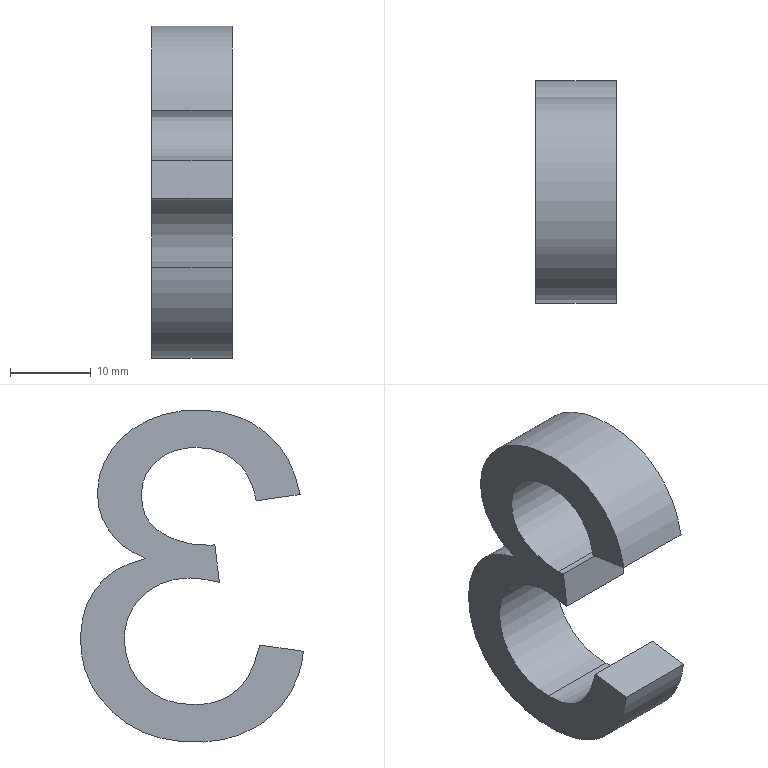Part | NX | features solid 2 | 1 solid | 14 faces | box 10 x 27.61 x 41.147 mm | volume 4412 mm3 | spline 9 | plane 5
STEP:
#1=CARTESIAN_POINT('',(2250.,-298.625,-587.676));
#2=VERTEX_POINT('',#1);
#3=CARTESIAN_POINT('',(2250.,-302.8,-579.522));
#4=VERTEX_POINT('',#3);
#5=CARTESIAN_POINT('',(2250.,-298.625,-587.676));
#6=CARTESIAN_POINT('',(2250.,-301.072,-585.595));
#7=CARTESIAN_POINT('',(2250.,-302.463,-582.872));
#8=CARTESIAN_POINT('',(2250.,-302.8,-579.522));
#9=B_SPLINE_CURVE_WITH_KNOTS('',3,(#5,#6,#7,#8),.UNSPECIFIED.,.F.,.F.,(4,4),(0.,0.04757),.PIECEWISE_BEZIER_KNOTS.);
#10=EDGE_CURVE('',#2,#4,#9,.T.);
#11=ORIENTED_EDGE('',*,*,#10,.F.);
#12=CARTESIAN_POINT('',(2260.,-298.625,-587.676));
#13=VERTEX_POINT('',#12);
#14=CARTESIAN_POINT('',(2260.,-298.625,-587.676));
#15=DIRECTION('',(-1.,0.,0.));
#16=VECTOR('',#15,1000.);
#17=LINE('',#14,#16);
#18=EDGE_CURVE('',#13,#2,#17,.T.);
#19=ORIENTED_EDGE('',*,*,#18,.F.);
#20=CARTESIAN_POINT('',(2260.,-302.8,-579.522));
#21=VERTEX_POINT('',#20);
#22=CARTESIAN_POINT('',(2260.,-298.625,-587.676));
#23=CARTESIAN_POINT('',(2260.,-301.072,-585.595));
#24=CARTESIAN_POINT('',(2260.,-302.463,-582.872));
#25=CARTESIAN_POINT('',(2260.,-302.8,-579.522));
#26=B_SPLINE_CURVE_WITH_KNOTS('',3,(#22,#23,#24,#25),.UNSPECIFIED.,.F.,.F.,(4,4),(0.,0.04757),.PIECEWISE_BEZIER_KNOTS.);
#27=EDGE_CURVE('',#13,#21,#26,.T.);
#28=ORIENTED_EDGE('',*,*,#27,.T.);
#29=CARTESIAN_POINT('',(2260.,-302.8,-579.522));
#30=DIRECTION('',(-1.,0.,0.));
#31=VECTOR('',#30,1000.);
#32=LINE('',#29,#31);
#33=EDGE_CURVE('',#21,#4,#32,.T.);
#34=ORIENTED_EDGE('',*,*,#33,.T.);
#35=EDGE_LOOP('',(#11,#19,#28,#34));
#36=FACE_BOUND('',#35,.T.);
#37=CARTESIAN_POINT('',(2260.,-298.625,-587.676));
#38=CARTESIAN_POINT('',(2250.,-298.625,-587.676));
#39=CARTESIAN_POINT('',(2260.,-301.072,-585.595));
#40=CARTESIAN_POINT('',(2250.,-301.072,-585.595));
#41=CARTESIAN_POINT('',(2260.,-302.463,-582.872));
#42=CARTESIAN_POINT('',(2250.,-302.463,-582.872));
#43=CARTESIAN_POINT('',(2260.,-302.8,-579.522));
#44=CARTESIAN_POINT('',(2250.,-302.8,-579.522));
#45=B_SPLINE_SURFACE_WITH_KNOTS('',3,1,((#37,#38),(#39,#40),(#41,#42),(#43,#44)),.SURF_OF_LINEAR_EXTRUSION.,.F.,.F.,.F.,(4,4),(2,2),(0.,0.04757),(0.,1.),.PIECEWISE_BEZIER_KNOTS.);
#46=ADVANCED_FACE('',(#36),#45,.T.);
#47=CARTESIAN_POINT('',(2250.,-297.37,-578.742));
#48=VERTEX_POINT('',#47);
#49=CARTESIAN_POINT('',(2250.,-302.8,-579.522));
#50=CARTESIAN_POINT('',(2250.,-300.99,-579.262));
#51=CARTESIAN_POINT('',(2250.,-299.18,-579.002));
#52=CARTESIAN_POINT('',(2250.,-297.37,-578.742));
#53=B_SPLINE_CURVE_WITH_KNOTS('',3,(#49,#50,#51,#52),.UNSPECIFIED.,.F.,.F.,(4,4),(0.04757,0.07533),.PIECEWISE_BEZIER_KNOTS.);
#54=EDGE_CURVE('',#4,#48,#53,.T.);
#55=ORIENTED_EDGE('',*,*,#54,.F.);
#56=ORIENTED_EDGE('',*,*,#33,.F.);
#57=CARTESIAN_POINT('',(2260.,-297.37,-578.742));
#58=VERTEX_POINT('',#57);
#59=CARTESIAN_POINT('',(2260.,-302.8,-579.522));
#60=CARTESIAN_POINT('',(2260.,-300.99,-579.262));
#61=CARTESIAN_POINT('',(2260.,-299.18,-579.002));
#62=CARTESIAN_POINT('',(2260.,-297.37,-578.742));
#63=B_SPLINE_CURVE_WITH_KNOTS('',3,(#59,#60,#61,#62),.UNSPECIFIED.,.F.,.F.,(4,4),(0.04757,0.07533),.PIECEWISE_BEZIER_KNOTS.);
#64=EDGE_CURVE('',#21,#58,#63,.T.);
#65=ORIENTED_EDGE('',*,*,#64,.T.);
#66=CARTESIAN_POINT('',(2260.,-297.37,-578.742));
#67=DIRECTION('',(-1.,0.,0.));
#68=VECTOR('',#67,1000.);
#69=LINE('',#66,#68);
#70=EDGE_CURVE('',#58,#48,#69,.T.);
#71=ORIENTED_EDGE('',*,*,#70,.T.);
#72=EDGE_LOOP('',(#55,#56,#65,#71));
#73=FACE_BOUND('',#72,.T.);
#74=CARTESIAN_POINT('',(2260.,-302.8,-579.522));
#75=DIRECTION('',(0.,-0.1422,0.9898));
#76=DIRECTION('',(0.,-0.9898,-0.1422));
#77=AXIS2_PLACEMENT_3D('',#74,#75,#76);
#78=PLANE('',#77);
#79=ADVANCED_FACE('',(#73),#78,.T.);
#80=CARTESIAN_POINT('',(2250.,-289.232,-586.115));
#81=VERTEX_POINT('',#80);
#82=CARTESIAN_POINT('',(2250.,-297.37,-578.742));
#83=CARTESIAN_POINT('',(2250.,-296.789,-581.388));
#84=CARTESIAN_POINT('',(2250.,-295.825,-583.285));
#85=CARTESIAN_POINT('',(2250.,-293.123,-585.583));
#86=CARTESIAN_POINT('',(2250.,-291.374,-586.145));
#87=CARTESIAN_POINT('',(2250.,-289.232,-586.115));
#88=B_SPLINE_CURVE_WITH_KNOTS('',3,(#82,#83,#84,#85,#86,#87),.UNSPECIFIED.,.F.,.F.,(4,2,4),(0.07533,0.1081,0.1418),.UNSPECIFIED.);
#89=EDGE_CURVE('',#48,#81,#88,.T.);
#90=ORIENTED_EDGE('',*,*,#89,.F.);
#91=ORIENTED_EDGE('',*,*,#70,.F.);
#92=CARTESIAN_POINT('',(2260.,-289.232,-586.115));
#93=VERTEX_POINT('',#92);
#94=CARTESIAN_POINT('',(2260.,-297.37,-578.742));
#95=CARTESIAN_POINT('',(2260.,-296.789,-581.388));
#96=CARTESIAN_POINT('',(2260.,-295.825,-583.285));
#97=CARTESIAN_POINT('',(2260.,-293.123,-585.583));
#98=CARTESIAN_POINT('',(2260.,-291.374,-586.145));
#99=CARTESIAN_POINT('',(2260.,-289.232,-586.115));
#100=B_SPLINE_CURVE_WITH_KNOTS('',3,(#94,#95,#96,#97,#98,#99),.UNSPECIFIED.,.F.,.F.,(4,2,4),(0.07533,0.1081,0.1418),.UNSPECIFIED.);
#101=EDGE_CURVE('',#58,#93,#100,.T.);
#102=ORIENTED_EDGE('',*,*,#101,.T.);
#103=CARTESIAN_POINT('',(2260.,-289.232,-586.115));
#104=DIRECTION('',(-1.,0.,0.));
#105=VECTOR('',#104,1000.);
#106=LINE('',#103,#105);
#107=EDGE_CURVE('',#93,#81,#106,.T.);
#108=ORIENTED_EDGE('',*,*,#107,.T.);
#109=EDGE_LOOP('',(#90,#91,#102,#108));
#110=FACE_BOUND('',#109,.T.);
#111=CARTESIAN_POINT('',(2260.,-297.37,-578.742));
#112=CARTESIAN_POINT('',(2250.,-297.37,-578.742));
#113=CARTESIAN_POINT('',(2260.,-296.19,-584.115));
#114=CARTESIAN_POINT('',(2250.,-296.19,-584.115));
#115=CARTESIAN_POINT('',(2260.,-293.452,-586.175));
#116=CARTESIAN_POINT('',(2250.,-293.452,-586.175));
#117=CARTESIAN_POINT('',(2260.,-289.232,-586.115));
#118=CARTESIAN_POINT('',(2250.,-289.232,-586.115));
#119=B_SPLINE_SURFACE_WITH_KNOTS('',3,1,((#111,#112),(#113,#114),(#115,#116),(#117,#118)),.SURF_OF_LINEAR_EXTRUSION.,.F.,.F.,.F.,(4,4),(2,2),(0.07533,0.1418),(0.,1.),.PIECEWISE_BEZIER_KNOTS.);
#120=ADVANCED_FACE('',(#110),#119,.T.);
#121=CARTESIAN_POINT('',(2250.,-288.789,-570.436));
#122=VERTEX_POINT('',#121);
#123=CARTESIAN_POINT('',(2250.,-289.232,-586.115));
#124=CARTESIAN_POINT('',(2250.,-286.678,-586.145));
#125=CARTESIAN_POINT('',(2250.,-284.613,-585.365));
#126=CARTESIAN_POINT('',(2250.,-283.014,-583.813));
#127=CARTESIAN_POINT('',(2250.,-281.416,-582.26));
#128=CARTESIAN_POINT('',(2250.,-280.636,-580.348));
#129=CARTESIAN_POINT('',(2250.,-280.636,-575.836));
#130=CARTESIAN_POINT('',(2250.,-281.385,-574.031));
#131=CARTESIAN_POINT('',(2250.,-284.451,-571.208));
#132=CARTESIAN_POINT('',(2250.,-286.418,-570.467));
#133=CARTESIAN_POINT('',(2250.,-288.789,-570.436));
#134=B_SPLINE_CURVE_WITH_KNOTS('',3,(#123,#124,#125,#126,#127,#128,#129,#130,#131,#132,#133),.UNSPECIFIED.,.F.,.F.,(4,3,2,2,4),(0.1418,0.1776,0.2115,0.243,0.2739),.UNSPECIFIED.);
#135=EDGE_CURVE('',#81,#122,#134,.T.);
#136=ORIENTED_EDGE('',*,*,#135,.F.);
#137=ORIENTED_EDGE('',*,*,#107,.F.);
#138=CARTESIAN_POINT('',(2260.,-288.789,-570.436));
#139=VERTEX_POINT('',#138);
#140=CARTESIAN_POINT('',(2260.,-289.232,-586.115));
#141=CARTESIAN_POINT('',(2260.,-286.678,-586.145));
#142=CARTESIAN_POINT('',(2260.,-284.613,-585.365));
#143=CARTESIAN_POINT('',(2260.,-283.014,-583.813));
#144=CARTESIAN_POINT('',(2260.,-281.416,-582.26));
#145=CARTESIAN_POINT('',(2260.,-280.636,-580.348));
#146=CARTESIAN_POINT('',(2260.,-280.636,-575.836));
#147=CARTESIAN_POINT('',(2260.,-281.385,-574.031));
#148=CARTESIAN_POINT('',(2260.,-284.451,-571.208));
#149=CARTESIAN_POINT('',(2260.,-286.418,-570.467));
#150=CARTESIAN_POINT('',(2260.,-288.789,-570.436));
#151=B_SPLINE_CURVE_WITH_KNOTS('',3,(#140,#141,#142,#143,#144,#145,#146,#147,#148,#149,#150),.UNSPECIFIED.,.F.,.F.,(4,3,2,2,4),(0.1418,0.1776,0.2115,0.243,0.2739),.UNSPECIFIED.);
#152=EDGE_CURVE('',#93,#139,#151,.T.);
#153=ORIENTED_EDGE('',*,*,#152,.T.);
#154=CARTESIAN_POINT('',(2260.,-288.789,-570.436));
#155=DIRECTION('',(-1.,0.,0.));
#156=VECTOR('',#155,1000.);
#157=LINE('',#154,#156);
#158=EDGE_CURVE('',#139,#122,#157,.T.);
#159=ORIENTED_EDGE('',*,*,#158,.T.);
#160=EDGE_LOOP('',(#136,#137,#153,#159));
#161=FACE_BOUND('',#160,.T.);
#162=CARTESIAN_POINT('',(2260.,-289.232,-586.115));
#163=CARTESIAN_POINT('',(2250.,-289.232,-586.115));
#164=CARTESIAN_POINT('',(2260.,-286.874,-586.143));
#165=CARTESIAN_POINT('',(2250.,-286.874,-586.143));
#166=CARTESIAN_POINT('',(2260.,-283.972,-585.165));
#167=CARTESIAN_POINT('',(2250.,-283.972,-585.165));
#168=CARTESIAN_POINT('',(2260.,-281.259,-581.812));
#169=CARTESIAN_POINT('',(2250.,-281.259,-581.812));
#170=CARTESIAN_POINT('',(2260.,-280.613,-579.348));
#171=CARTESIAN_POINT('',(2250.,-280.613,-579.348));
#172=CARTESIAN_POINT('',(2260.,-280.632,-577.039));
#173=CARTESIAN_POINT('',(2250.,-280.632,-577.039));
#174=CARTESIAN_POINT('',(2260.,-281.071,-574.988));
#175=CARTESIAN_POINT('',(2250.,-281.071,-574.988));
#176=CARTESIAN_POINT('',(2260.,-282.446,-572.761));
#177=CARTESIAN_POINT('',(2250.,-282.446,-572.761));
#178=CARTESIAN_POINT('',(2260.,-285.243,-570.874));
#179=CARTESIAN_POINT('',(2250.,-285.243,-570.874));
#180=CARTESIAN_POINT('',(2260.,-287.524,-570.452));
#181=CARTESIAN_POINT('',(2250.,-287.524,-570.452));
#182=CARTESIAN_POINT('',(2260.,-288.789,-570.436));
#183=CARTESIAN_POINT('',(2250.,-288.789,-570.436));
#184=B_SPLINE_SURFACE_WITH_KNOTS('',3,1,((#162,#163),(#164,#165),(#166,#167),(#168,#169),(#170,#171),(#172,#173),(#174,#175),(#176,#177),(#178,#179),(#180,#181),(#182,#183)),.SURF_OF_LINEAR_EXTRUSION.,.F.,.F.,.F.,(4,1,1,1,1,1,1,1,4),(2,2),(0.1418,0.1748,0.1914,0.2079,0.2161,0.2244,0.2409,0.2574,0.2739),(0.,1.),.UNSPECIFIED.);
#185=ADVANCED_FACE('',(#161),#184,.T.);
#186=CARTESIAN_POINT('',(2250.,-292.398,-570.971));
#187=VERTEX_POINT('',#186);
#188=CARTESIAN_POINT('',(2250.,-288.789,-570.436));
#189=CARTESIAN_POINT('',(2250.,-289.752,-570.467));
#190=CARTESIAN_POINT('',(2250.,-290.961,-570.635));
#191=CARTESIAN_POINT('',(2250.,-292.398,-570.971));
#192=B_SPLINE_CURVE_WITH_KNOTS('',3,(#188,#189,#190,#191),.UNSPECIFIED.,.F.,.F.,(4,4),(0.2739,0.2929),.PIECEWISE_BEZIER_KNOTS.);
#193=EDGE_CURVE('',#122,#187,#192,.T.);
#194=ORIENTED_EDGE('',*,*,#193,.F.);
#195=ORIENTED_EDGE('',*,*,#158,.F.);
#196=CARTESIAN_POINT('',(2260.,-292.398,-570.971));
#197=VERTEX_POINT('',#196);
#198=CARTESIAN_POINT('',(2260.,-288.789,-570.436));
#199=CARTESIAN_POINT('',(2260.,-289.752,-570.467));
#200=CARTESIAN_POINT('',(2260.,-290.961,-570.635));
#201=CARTESIAN_POINT('',(2260.,-292.398,-570.971));
#202=B_SPLINE_CURVE_WITH_KNOTS('',3,(#198,#199,#200,#201),.UNSPECIFIED.,.F.,.F.,(4,4),(0.2739,0.2929),.PIECEWISE_BEZIER_KNOTS.);
#203=EDGE_CURVE('',#139,#197,#202,.T.);
#204=ORIENTED_EDGE('',*,*,#203,.T.);
#205=CARTESIAN_POINT('',(2260.,-292.398,-570.971));
#206=DIRECTION('',(-1.,0.,0.));
#207=VECTOR('',#206,1000.);
#208=LINE('',#205,#207);
#209=EDGE_CURVE('',#197,#187,#208,.T.);
#210=ORIENTED_EDGE('',*,*,#209,.T.);
#211=EDGE_LOOP('',(#194,#195,#204,#210));
#212=FACE_BOUND('',#211,.T.);
#213=CARTESIAN_POINT('',(2260.,-288.789,-570.436));
#214=CARTESIAN_POINT('',(2250.,-288.789,-570.436));
#215=CARTESIAN_POINT('',(2260.,-289.752,-570.467));
#216=CARTESIAN_POINT('',(2250.,-289.752,-570.467));
#217=CARTESIAN_POINT('',(2260.,-290.961,-570.635));
#218=CARTESIAN_POINT('',(2250.,-290.961,-570.635));
#219=CARTESIAN_POINT('',(2260.,-292.398,-570.971));
#220=CARTESIAN_POINT('',(2250.,-292.398,-570.971));
#221=B_SPLINE_SURFACE_WITH_KNOTS('',3,1,((#213,#214),(#215,#216),(#217,#218),(#219,#220)),.SURF_OF_LINEAR_EXTRUSION.,.F.,.F.,.F.,(4,4),(2,2),(0.2739,0.2929),(0.,1.),.PIECEWISE_BEZIER_KNOTS.);
#222=ADVANCED_FACE('',(#212),#221,.T.);
#223=CARTESIAN_POINT('',(2250.,-291.817,-566.321));
#224=VERTEX_POINT('',#223);
#225=CARTESIAN_POINT('',(2250.,-292.398,-570.971));
#226=CARTESIAN_POINT('',(2250.,-292.205,-569.421));
#227=CARTESIAN_POINT('',(2250.,-292.011,-567.871));
#228=CARTESIAN_POINT('',(2250.,-291.817,-566.321));
#229=B_SPLINE_CURVE_WITH_KNOTS('',3,(#225,#226,#227,#228),.UNSPECIFIED.,.F.,.F.,(4,4),(0.2929,0.3173),.PIECEWISE_BEZIER_KNOTS.);
#230=EDGE_CURVE('',#187,#224,#229,.T.);
#231=ORIENTED_EDGE('',*,*,#230,.F.);
#232=ORIENTED_EDGE('',*,*,#209,.F.);
#233=CARTESIAN_POINT('',(2260.,-291.817,-566.321));
#234=VERTEX_POINT('',#233);
#235=CARTESIAN_POINT('',(2260.,-292.398,-570.971));
#236=CARTESIAN_POINT('',(2260.,-292.205,-569.421));
#237=CARTESIAN_POINT('',(2260.,-292.011,-567.871));
#238=CARTESIAN_POINT('',(2260.,-291.817,-566.321));
#239=B_SPLINE_CURVE_WITH_KNOTS('',3,(#235,#236,#237,#238),.UNSPECIFIED.,.F.,.F.,(4,4),(0.2929,0.3173),.PIECEWISE_BEZIER_KNOTS.);
#240=EDGE_CURVE('',#197,#234,#239,.T.);
#241=ORIENTED_EDGE('',*,*,#240,.T.);
#242=CARTESIAN_POINT('',(2260.,-291.817,-566.321));
#243=DIRECTION('',(-1.,0.,0.));
#244=VECTOR('',#243,1000.);
#245=LINE('',#242,#244);
#246=EDGE_CURVE('',#234,#224,#245,.T.);
#247=ORIENTED_EDGE('',*,*,#246,.T.);
#248=EDGE_LOOP('',(#231,#232,#241,#247));
#249=FACE_BOUND('',#248,.T.);
#250=CARTESIAN_POINT('',(2260.,-292.398,-570.971));
#251=DIRECTION('',(0.,-0.9923,0.124));
#252=DIRECTION('',(0.,-0.124,-0.9923));
#253=AXIS2_PLACEMENT_3D('',#250,#251,#252);
#254=PLANE('',#253);
#255=ADVANCED_FACE('',(#249),#254,.T.);
#256=CARTESIAN_POINT('',(2250.,-291.007,-566.382));
#257=VERTEX_POINT('',#256);
#258=CARTESIAN_POINT('',(2250.,-291.817,-566.321));
#259=CARTESIAN_POINT('',(2250.,-291.481,-566.382));
#260=CARTESIAN_POINT('',(2250.,-291.221,-566.413));
#261=CARTESIAN_POINT('',(2250.,-291.007,-566.382));
#262=B_SPLINE_CURVE_WITH_KNOTS('',3,(#258,#259,#260,#261),.UNSPECIFIED.,.F.,.F.,(4,4),(0.3173,0.3215),.PIECEWISE_BEZIER_KNOTS.);
#263=EDGE_CURVE('',#224,#257,#262,.T.);
#264=ORIENTED_EDGE('',*,*,#263,.F.);
#265=ORIENTED_EDGE('',*,*,#246,.F.);
#266=CARTESIAN_POINT('',(2260.,-291.007,-566.382));
#267=VERTEX_POINT('',#266);
#268=CARTESIAN_POINT('',(2260.,-291.817,-566.321));
#269=CARTESIAN_POINT('',(2260.,-291.481,-566.382));
#270=CARTESIAN_POINT('',(2260.,-291.221,-566.413));
#271=CARTESIAN_POINT('',(2260.,-291.007,-566.382));
#272=B_SPLINE_CURVE_WITH_KNOTS('',3,(#268,#269,#270,#271),.UNSPECIFIED.,.F.,.F.,(4,4),(0.3173,0.3215),.PIECEWISE_BEZIER_KNOTS.);
#273=EDGE_CURVE('',#234,#267,#272,.T.);
#274=ORIENTED_EDGE('',*,*,#273,.T.);
#275=CARTESIAN_POINT('',(2260.,-291.007,-566.382));
#276=DIRECTION('',(-1.,0.,0.));
#277=VECTOR('',#276,1000.);
#278=LINE('',#275,#277);
#279=EDGE_CURVE('',#267,#257,#278,.T.);
#280=ORIENTED_EDGE('',*,*,#279,.T.);
#281=EDGE_LOOP('',(#264,#265,#274,#280));
#282=FACE_BOUND('',#281,.T.);
#283=CARTESIAN_POINT('',(2260.,-291.817,-566.321));
#284=CARTESIAN_POINT('',(2250.,-291.817,-566.321));
#285=CARTESIAN_POINT('',(2260.,-291.481,-566.382));
#286=CARTESIAN_POINT('',(2250.,-291.481,-566.382));
#287=CARTESIAN_POINT('',(2260.,-291.221,-566.413));
#288=CARTESIAN_POINT('',(2250.,-291.221,-566.413));
#289=CARTESIAN_POINT('',(2260.,-291.007,-566.382));
#290=CARTESIAN_POINT('',(2250.,-291.007,-566.382));
#291=B_SPLINE_SURFACE_WITH_KNOTS('',3,1,((#283,#284),(#285,#286),(#287,#288),(#289,#290)),.SURF_OF_LINEAR_EXTRUSION.,.F.,.F.,.F.,(4,4),(2,2),(0.3173,0.3215),(0.,1.),.PIECEWISE_BEZIER_KNOTS.);
#292=ADVANCED_FACE('',(#282),#291,.T.);
#293=CARTESIAN_POINT('',(2250.,-289.492,-554.268));
#294=VERTEX_POINT('',#293);
#295=CARTESIAN_POINT('',(2250.,-291.007,-566.382));
#296=CARTESIAN_POINT('',(2250.,-288.865,-566.413));
#297=CARTESIAN_POINT('',(2250.,-286.968,-565.908));
#298=CARTESIAN_POINT('',(2250.,-285.247,-564.866));
#299=CARTESIAN_POINT('',(2250.,-283.557,-563.843));
#300=CARTESIAN_POINT('',(2250.,-282.731,-562.268));
#301=CARTESIAN_POINT('',(2250.,-282.731,-558.474));
#302=CARTESIAN_POINT('',(2250.,-283.358,-557.067));
#303=CARTESIAN_POINT('',(2250.,-284.62,-555.959));
#304=CARTESIAN_POINT('',(2250.,-285.867,-554.864));
#305=CARTESIAN_POINT('',(2250.,-287.504,-554.298));
#306=CARTESIAN_POINT('',(2250.,-289.492,-554.268));
#307=B_SPLINE_CURVE_WITH_KNOTS('',3,(#295,#296,#297,#298,#299,#300,#301,#302,#303,#304,#305,#306),.UNSPECIFIED.,.F.,.F.,(4,3,2,3,4),(0.3215,0.3528,0.3821,0.4047,0.4319),.UNSPECIFIED.);
#308=EDGE_CURVE('',#257,#294,#307,.T.);
#309=ORIENTED_EDGE('',*,*,#308,.F.);
#310=ORIENTED_EDGE('',*,*,#279,.F.);
#311=CARTESIAN_POINT('',(2260.,-289.492,-554.268));
#312=VERTEX_POINT('',#311);
#313=CARTESIAN_POINT('',(2260.,-291.007,-566.382));
#314=CARTESIAN_POINT('',(2260.,-288.865,-566.413));
#315=CARTESIAN_POINT('',(2260.,-286.968,-565.908));
#316=CARTESIAN_POINT('',(2260.,-285.247,-564.866));
#317=CARTESIAN_POINT('',(2260.,-283.557,-563.843));
#318=CARTESIAN_POINT('',(2260.,-282.731,-562.268));
#319=CARTESIAN_POINT('',(2260.,-282.731,-558.474));
#320=CARTESIAN_POINT('',(2260.,-283.358,-557.067));
#321=CARTESIAN_POINT('',(2260.,-284.62,-555.959));
#322=CARTESIAN_POINT('',(2260.,-285.867,-554.864));
#323=CARTESIAN_POINT('',(2260.,-287.504,-554.298));
#324=CARTESIAN_POINT('',(2260.,-289.492,-554.268));
#325=B_SPLINE_CURVE_WITH_KNOTS('',3,(#313,#314,#315,#316,#317,#318,#319,#320,#321,#322,#323,#324),.UNSPECIFIED.,.F.,.F.,(4,3,2,3,4),(0.3215,0.3528,0.3821,0.4047,0.4319),.UNSPECIFIED.);
#326=EDGE_CURVE('',#267,#312,#325,.T.);
#327=ORIENTED_EDGE('',*,*,#326,.T.);
#328=CARTESIAN_POINT('',(2260.,-289.492,-554.268));
#329=DIRECTION('',(-1.,0.,0.));
#330=VECTOR('',#329,1000.);
#331=LINE('',#328,#330);
#332=EDGE_CURVE('',#312,#294,#331,.T.);
#333=ORIENTED_EDGE('',*,*,#332,.T.);
#334=EDGE_LOOP('',(#309,#310,#327,#333));
#335=FACE_BOUND('',#334,.T.);
#336=CARTESIAN_POINT('',(2260.,-291.007,-566.382));
#337=CARTESIAN_POINT('',(2250.,-291.007,-566.382));
#338=CARTESIAN_POINT('',(2260.,-290.063,-566.396));
#339=CARTESIAN_POINT('',(2250.,-290.063,-566.396));
#340=CARTESIAN_POINT('',(2260.,-288.271,-566.21));
#341=CARTESIAN_POINT('',(2250.,-288.271,-566.21));
#342=CARTESIAN_POINT('',(2260.,-285.84,-565.338));
#343=CARTESIAN_POINT('',(2250.,-285.84,-565.338));
#344=CARTESIAN_POINT('',(2260.,-283.591,-563.735));
#345=CARTESIAN_POINT('',(2250.,-283.591,-563.735));
#346=CARTESIAN_POINT('',(2260.,-282.803,-561.792));
#347=CARTESIAN_POINT('',(2250.,-282.803,-561.792));
#348=CARTESIAN_POINT('',(2260.,-282.683,-559.786));
#349=CARTESIAN_POINT('',(2250.,-282.683,-559.786));
#350=CARTESIAN_POINT('',(2260.,-282.932,-558.358));
#351=CARTESIAN_POINT('',(2250.,-282.932,-558.358));
#352=CARTESIAN_POINT('',(2260.,-283.442,-557.302));
#353=CARTESIAN_POINT('',(2250.,-283.442,-557.302));
#354=CARTESIAN_POINT('',(2260.,-284.014,-556.543));
#355=CARTESIAN_POINT('',(2250.,-284.014,-556.543));
#356=CARTESIAN_POINT('',(2260.,-284.753,-555.803));
#357=CARTESIAN_POINT('',(2250.,-284.753,-555.803));
#358=CARTESIAN_POINT('',(2260.,-285.547,-555.242));
#359=CARTESIAN_POINT('',(2250.,-285.547,-555.242));
#360=CARTESIAN_POINT('',(2260.,-287.117,-554.504));
#361=CARTESIAN_POINT('',(2250.,-287.117,-554.504));
#362=CARTESIAN_POINT('',(2260.,-288.485,-554.283));
#363=CARTESIAN_POINT('',(2250.,-288.485,-554.283));
#364=CARTESIAN_POINT('',(2260.,-289.492,-554.268));
#365=CARTESIAN_POINT('',(2250.,-289.492,-554.268));
#366=B_SPLINE_SURFACE_WITH_KNOTS('',3,1,((#336,#337),(#338,#339),(#340,#341),(#342,#343),(#344,#345),(#346,#347),(#348,#349),(#350,#351),(#352,#353),(#354,#355),(#356,#357),(#358,#359),(#360,#361),(#362,#363),(#364,#365)),.SURF_OF_LINEAR_EXTRUSION.,.F.,.F.,.F.,(4,1,1,1,1,1,1,1,1,1,1,1,4),(2,2),(0.3215,0.3353,0.3491,0.3629,0.3767,0.3836,0.3905,0.3974,0.4009,0.4043,0.4112,0.4181,0.4319),(0.,1.),.UNSPECIFIED.);
#367=ADVANCED_FACE('',(#335),#366,.T.);
#368=CARTESIAN_POINT('',(2250.,-296.941,-560.876));
#369=VERTEX_POINT('',#368);
#370=CARTESIAN_POINT('',(2250.,-289.492,-554.268));
#371=CARTESIAN_POINT('',(2250.,-291.45,-554.298));
#372=CARTESIAN_POINT('',(2250.,-293.102,-554.864));
#373=CARTESIAN_POINT('',(2250.,-294.407,-555.963));
#374=CARTESIAN_POINT('',(2250.,-295.718,-557.067));
#375=CARTESIAN_POINT('',(2250.,-296.574,-558.688));
#376=CARTESIAN_POINT('',(2250.,-296.941,-560.876));
#377=B_SPLINE_CURVE_WITH_KNOTS('',3,(#370,#371,#372,#373,#374,#375,#376),.UNSPECIFIED.,.F.,.F.,(4,3,4),(0.4319,0.4594,0.4886),.PIECEWISE_BEZIER_KNOTS.);
#378=EDGE_CURVE('',#294,#369,#377,.T.);
#379=ORIENTED_EDGE('',*,*,#378,.F.);
#380=ORIENTED_EDGE('',*,*,#332,.F.);
#381=CARTESIAN_POINT('',(2260.,-296.941,-560.876));
#382=VERTEX_POINT('',#381);
#383=CARTESIAN_POINT('',(2260.,-289.492,-554.268));
#384=CARTESIAN_POINT('',(2260.,-291.45,-554.298));
#385=CARTESIAN_POINT('',(2260.,-293.102,-554.864));
#386=CARTESIAN_POINT('',(2260.,-294.407,-555.963));
#387=CARTESIAN_POINT('',(2260.,-295.718,-557.067));
#388=CARTESIAN_POINT('',(2260.,-296.574,-558.688));
#389=CARTESIAN_POINT('',(2260.,-296.941,-560.876));
#390=B_SPLINE_CURVE_WITH_KNOTS('',3,(#383,#384,#385,#386,#387,#388,#389),.UNSPECIFIED.,.F.,.F.,(4,3,4),(0.4319,0.4594,0.4886),.PIECEWISE_BEZIER_KNOTS.);
#391=EDGE_CURVE('',#312,#382,#390,.T.);
#392=ORIENTED_EDGE('',*,*,#391,.T.);
#393=CARTESIAN_POINT('',(2260.,-296.941,-560.876));
#394=DIRECTION('',(-1.,0.,0.));
#395=VECTOR('',#394,1000.);
#396=LINE('',#393,#395);
#397=EDGE_CURVE('',#382,#369,#396,.T.);
#398=ORIENTED_EDGE('',*,*,#397,.T.);
#399=EDGE_LOOP('',(#379,#380,#392,#398));
#400=FACE_BOUND('',#399,.T.);
#401=CARTESIAN_POINT('',(2260.,-289.492,-554.268));
#402=CARTESIAN_POINT('',(2250.,-289.492,-554.268));
#403=CARTESIAN_POINT('',(2260.,-290.503,-554.283));
#404=CARTESIAN_POINT('',(2250.,-290.503,-554.283));
#405=CARTESIAN_POINT('',(2260.,-292.354,-554.593));
#406=CARTESIAN_POINT('',(2250.,-292.354,-554.593));
#407=CARTESIAN_POINT('',(2260.,-295.415,-556.41));
#408=CARTESIAN_POINT('',(2250.,-295.415,-556.41));
#409=CARTESIAN_POINT('',(2260.,-296.586,-558.755));
#410=CARTESIAN_POINT('',(2250.,-296.586,-558.755));
#411=CARTESIAN_POINT('',(2260.,-296.941,-560.876));
#412=CARTESIAN_POINT('',(2250.,-296.941,-560.876));
#413=B_SPLINE_SURFACE_WITH_KNOTS('',3,1,((#401,#402),(#403,#404),(#405,#406),(#407,#408),(#409,#410),(#411,#412)),.SURF_OF_LINEAR_EXTRUSION.,.F.,.F.,.F.,(4,1,1,4),(2,2),(0.4319,0.4461,0.4602,0.4886),(0.,1.),.UNSPECIFIED.);
#414=ADVANCED_FACE('',(#400),#413,.T.);
#415=CARTESIAN_POINT('',(2250.,-302.387,-560.096));
#416=VERTEX_POINT('',#415);
#417=CARTESIAN_POINT('',(2250.,-296.941,-560.876));
#418=CARTESIAN_POINT('',(2250.,-298.757,-560.616));
#419=CARTESIAN_POINT('',(2250.,-300.572,-560.356));
#420=CARTESIAN_POINT('',(2250.,-302.387,-560.096));
#421=B_SPLINE_CURVE_WITH_KNOTS('',3,(#417,#418,#419,#420),.UNSPECIFIED.,.F.,.F.,(4,4),(0.4886,0.517),.PIECEWISE_BEZIER_KNOTS.);
#422=EDGE_CURVE('',#369,#416,#421,.T.);
#423=ORIENTED_EDGE('',*,*,#422,.F.);
#424=ORIENTED_EDGE('',*,*,#397,.F.);
#425=CARTESIAN_POINT('',(2260.,-302.387,-560.096));
#426=VERTEX_POINT('',#425);
#427=CARTESIAN_POINT('',(2260.,-296.941,-560.876));
#428=CARTESIAN_POINT('',(2260.,-298.757,-560.616));
#429=CARTESIAN_POINT('',(2260.,-300.572,-560.356));
#430=CARTESIAN_POINT('',(2260.,-302.387,-560.096));
#431=B_SPLINE_CURVE_WITH_KNOTS('',3,(#427,#428,#429,#430),.UNSPECIFIED.,.F.,.F.,(4,4),(0.4886,0.517),.PIECEWISE_BEZIER_KNOTS.);
#432=EDGE_CURVE('',#382,#426,#431,.T.);
#433=ORIENTED_EDGE('',*,*,#432,.T.);
#434=CARTESIAN_POINT('',(2260.,-302.387,-560.096));
#435=DIRECTION('',(-1.,0.,0.));
#436=VECTOR('',#435,1000.);
#437=LINE('',#434,#436);
#438=EDGE_CURVE('',#426,#416,#437,.T.);
#439=ORIENTED_EDGE('',*,*,#438,.T.);
#440=EDGE_LOOP('',(#423,#424,#433,#439));
#441=FACE_BOUND('',#440,.T.);
#442=CARTESIAN_POINT('',(2260.,-296.941,-560.876));
#443=DIRECTION('',(0.,-0.1418,-0.9899));
#444=DIRECTION('',(0.,0.9899,-0.1418));
#445=AXIS2_PLACEMENT_3D('',#442,#443,#444);
#446=PLANE('',#445);
#447=ADVANCED_FACE('',(#441),#446,.T.);
#448=CARTESIAN_POINT('',(2250.,-283.251,-568.034));
#449=VERTEX_POINT('',#448);
#450=CARTESIAN_POINT('',(2250.,-302.387,-560.096));
#451=CARTESIAN_POINT('',(2250.,-301.76,-556.792));
#452=CARTESIAN_POINT('',(2250.,-300.322,-554.222));
#453=CARTESIAN_POINT('',(2250.,-295.832,-550.557));
#454=CARTESIAN_POINT('',(2250.,-293.026,-549.633));
#455=CARTESIAN_POINT('',(2250.,-289.676,-549.633));
#456=CARTESIAN_POINT('',(2250.,-287.351,-549.633));
#457=CARTESIAN_POINT('',(2250.,-285.209,-550.122));
#458=CARTESIAN_POINT('',(2250.,-283.286,-551.05));
#459=CARTESIAN_POINT('',(2250.,-281.339,-551.989));
#460=CARTESIAN_POINT('',(2250.,-279.855,-553.258));
#461=CARTESIAN_POINT('',(2250.,-277.794,-556.488));
#462=CARTESIAN_POINT('',(2250.,-277.286,-558.184));
#463=CARTESIAN_POINT('',(2250.,-277.286,-561.732));
#464=CARTESIAN_POINT('',(2250.,-277.79,-563.277));
#465=CARTESIAN_POINT('',(2250.,-279.779,-566.092));
#466=CARTESIAN_POINT('',(2250.,-281.263,-567.208));
#467=CARTESIAN_POINT('',(2250.,-283.251,-568.034));
#468=B_SPLINE_CURVE_WITH_KNOTS('',3,(#450,#451,#452,#453,#454,#455,#456,#457,#458,#459,#460,#461,#462,#463,#464,#465,#466,#467),.UNSPECIFIED.,.F.,.F.,(4,2,3,3,2,2,2,4),(0.517,0.5636,0.6101,0.6443,0.675,0.706,0.7366,0.7671),.UNSPECIFIED.);
#469=EDGE_CURVE('',#416,#449,#468,.T.);
#470=ORIENTED_EDGE('',*,*,#469,.F.);
#471=ORIENTED_EDGE('',*,*,#438,.F.);
#472=CARTESIAN_POINT('',(2260.,-283.251,-568.034));
#473=VERTEX_POINT('',#472);
#474=CARTESIAN_POINT('',(2260.,-302.387,-560.096));
#475=CARTESIAN_POINT('',(2260.,-301.76,-556.792));
#476=CARTESIAN_POINT('',(2260.,-300.322,-554.222));
#477=CARTESIAN_POINT('',(2260.,-295.832,-550.557));
#478=CARTESIAN_POINT('',(2260.,-293.026,-549.633));
#479=CARTESIAN_POINT('',(2260.,-289.676,-549.633));
#480=CARTESIAN_POINT('',(2260.,-287.351,-549.633));
#481=CARTESIAN_POINT('',(2260.,-285.209,-550.122));
#482=CARTESIAN_POINT('',(2260.,-283.286,-551.05));
#483=CARTESIAN_POINT('',(2260.,-281.339,-551.989));
#484=CARTESIAN_POINT('',(2260.,-279.855,-553.258));
#485=CARTESIAN_POINT('',(2260.,-277.794,-556.488));
#486=CARTESIAN_POINT('',(2260.,-277.286,-558.184));
#487=CARTESIAN_POINT('',(2260.,-277.286,-561.732));
#488=CARTESIAN_POINT('',(2260.,-277.79,-563.277));
#489=CARTESIAN_POINT('',(2260.,-279.779,-566.092));
#490=CARTESIAN_POINT('',(2260.,-281.263,-567.208));
#491=CARTESIAN_POINT('',(2260.,-283.251,-568.034));
#492=B_SPLINE_CURVE_WITH_KNOTS('',3,(#474,#475,#476,#477,#478,#479,#480,#481,#482,#483,#484,#485,#486,#487,#488,#489,#490,#491),.UNSPECIFIED.,.F.,.F.,(4,2,3,3,2,2,2,4),(0.517,0.5636,0.6101,0.6443,0.675,0.706,0.7366,0.7671),.UNSPECIFIED.);
#493=EDGE_CURVE('',#426,#473,#492,.T.);
#494=ORIENTED_EDGE('',*,*,#493,.T.);
#495=CARTESIAN_POINT('',(2260.,-283.251,-568.034));
#496=DIRECTION('',(-1.,0.,0.));
#497=VECTOR('',#496,1000.);
#498=LINE('',#495,#497);
#499=EDGE_CURVE('',#473,#449,#498,.T.);
#500=ORIENTED_EDGE('',*,*,#499,.T.);
#501=EDGE_LOOP('',(#470,#471,#494,#500));
#502=FACE_BOUND('',#501,.T.);
#503=CARTESIAN_POINT('',(2260.,-302.387,-560.096));
#504=CARTESIAN_POINT('',(2250.,-302.387,-560.096));
#505=CARTESIAN_POINT('',(2260.,-301.967,-557.881));
#506=CARTESIAN_POINT('',(2250.,-301.967,-557.881));
#507=CARTESIAN_POINT('',(2260.,-300.799,-555.06));
#508=CARTESIAN_POINT('',(2250.,-300.799,-555.06));
#509=CARTESIAN_POINT('',(2260.,-298.114,-552.264));
#510=CARTESIAN_POINT('',(2250.,-298.114,-552.264));
#511=CARTESIAN_POINT('',(2260.,-295.641,-550.723));
#512=CARTESIAN_POINT('',(2250.,-295.641,-550.723));
#513=CARTESIAN_POINT('',(2260.,-293.275,-549.968));
#514=CARTESIAN_POINT('',(2250.,-293.275,-549.968));
#515=CARTESIAN_POINT('',(2260.,-291.207,-549.673));
#516=CARTESIAN_POINT('',(2250.,-291.207,-549.673));
#517=CARTESIAN_POINT('',(2260.,-288.963,-549.585));
#518=CARTESIAN_POINT('',(2250.,-288.963,-549.585));
#519=CARTESIAN_POINT('',(2260.,-286.429,-549.873));
#520=CARTESIAN_POINT('',(2250.,-286.429,-549.873));
#521=CARTESIAN_POINT('',(2260.,-283.671,-550.749));
#522=CARTESIAN_POINT('',(2250.,-283.671,-550.749));
#523=CARTESIAN_POINT('',(2260.,-280.861,-552.381));
#524=CARTESIAN_POINT('',(2250.,-280.861,-552.381));
#525=CARTESIAN_POINT('',(2260.,-278.218,-555.27));
#526=CARTESIAN_POINT('',(2250.,-278.218,-555.27));
#527=CARTESIAN_POINT('',(2260.,-277.047,-558.857));
#528=CARTESIAN_POINT('',(2250.,-277.047,-558.857));
#529=CARTESIAN_POINT('',(2260.,-277.48,-562.345));
#530=CARTESIAN_POINT('',(2250.,-277.48,-562.345));
#531=CARTESIAN_POINT('',(2260.,-278.954,-565.405));
#532=CARTESIAN_POINT('',(2250.,-278.954,-565.405));
#533=CARTESIAN_POINT('',(2260.,-281.215,-567.189));
#534=CARTESIAN_POINT('',(2250.,-281.215,-567.189));
#535=CARTESIAN_POINT('',(2260.,-283.251,-568.034));
#536=CARTESIAN_POINT('',(2250.,-283.251,-568.034));
#537=B_SPLINE_SURFACE_WITH_KNOTS('',3,1,((#503,#504),(#505,#506),(#507,#508),(#509,#510),(#511,#512),(#513,#514),(#515,#516),(#517,#518),(#519,#520),(#521,#522),(#523,#524),(#525,#526),(#527,#528),(#529,#530),(#531,#532),(#533,#534),(#535,#536)),.SURF_OF_LINEAR_EXTRUSION.,.F.,.F.,.F.,(4,1,1,1,1,1,1,1,1,1,1,1,1,1,4),(2,2),(0.517,0.5483,0.5639,0.5795,0.5952,0.603,0.6108,0.6264,0.642,0.6577,0.6733,0.7046,0.7202,0.7358,0.7671),(0.,1.),.UNSPECIFIED.);
#538=ADVANCED_FACE('',(#502),#537,.T.);
#539=CARTESIAN_POINT('',(2250.,-283.251,-568.034));
#540=CARTESIAN_POINT('',(2250.,-280.681,-568.616));
#541=CARTESIAN_POINT('',(2250.,-278.693,-569.763));
#542=CARTESIAN_POINT('',(2250.,-275.878,-573.25));
#543=CARTESIAN_POINT('',(2250.,-275.19,-575.438));
#544=CARTESIAN_POINT('',(2250.,-275.19,-581.633));
#545=CARTESIAN_POINT('',(2250.,-276.536,-584.646));
#546=CARTESIAN_POINT('',(2250.,-279.214,-587.11));
#547=CARTESIAN_POINT('',(2250.,-281.89,-589.572));
#548=CARTESIAN_POINT('',(2250.,-285.286,-590.78));
#549=CARTESIAN_POINT('',(2250.,-293.102,-590.78));
#550=CARTESIAN_POINT('',(2250.,-296.161,-589.771));
#551=CARTESIAN_POINT('',(2250.,-298.625,-587.676));
#552=B_SPLINE_CURVE_WITH_KNOTS('',3,(#539,#540,#541,#542,#543,#544,#545,#546,#547,#548,#549,#550,#551),.UNSPECIFIED.,.F.,.F.,(4,2,2,3,2,4),(0.7671,0.8039,0.8407,0.8905,0.9484,1.),.UNSPECIFIED.);
#553=EDGE_CURVE('',#449,#2,#552,.T.);
#554=ORIENTED_EDGE('',*,*,#553,.F.);
#555=ORIENTED_EDGE('',*,*,#499,.F.);
#556=CARTESIAN_POINT('',(2260.,-283.251,-568.034));
#557=CARTESIAN_POINT('',(2260.,-280.681,-568.616));
#558=CARTESIAN_POINT('',(2260.,-278.693,-569.763));
#559=CARTESIAN_POINT('',(2260.,-275.878,-573.25));
#560=CARTESIAN_POINT('',(2260.,-275.19,-575.438));
#561=CARTESIAN_POINT('',(2260.,-275.19,-581.633));
#562=CARTESIAN_POINT('',(2260.,-276.536,-584.646));
#563=CARTESIAN_POINT('',(2260.,-279.214,-587.11));
#564=CARTESIAN_POINT('',(2260.,-281.89,-589.572));
#565=CARTESIAN_POINT('',(2260.,-285.286,-590.78));
#566=CARTESIAN_POINT('',(2260.,-293.102,-590.78));
#567=CARTESIAN_POINT('',(2260.,-296.161,-589.771));
#568=CARTESIAN_POINT('',(2260.,-298.625,-587.676));
#569=B_SPLINE_CURVE_WITH_KNOTS('',3,(#556,#557,#558,#559,#560,#561,#562,#563,#564,#565,#566,#567,#568),.UNSPECIFIED.,.F.,.F.,(4,2,2,3,2,4),(0.7671,0.8039,0.8407,0.8905,0.9484,1.),.UNSPECIFIED.);
#570=EDGE_CURVE('',#473,#13,#569,.T.);
#571=ORIENTED_EDGE('',*,*,#570,.T.);
#572=ORIENTED_EDGE('',*,*,#18,.T.);
#573=EDGE_LOOP('',(#554,#555,#571,#572));
#574=FACE_BOUND('',#573,.T.);
#575=CARTESIAN_POINT('',(2260.,-283.251,-568.034));
#576=CARTESIAN_POINT('',(2250.,-283.251,-568.034));
#577=CARTESIAN_POINT('',(2260.,-281.218,-568.494));
#578=CARTESIAN_POINT('',(2250.,-281.218,-568.494));
#579=CARTESIAN_POINT('',(2260.,-278.719,-569.708));
#580=CARTESIAN_POINT('',(2250.,-278.719,-569.708));
#581=CARTESIAN_POINT('',(2260.,-276.459,-572.466));
#582=CARTESIAN_POINT('',(2250.,-276.459,-572.466));
#583=CARTESIAN_POINT('',(2260.,-275.444,-574.922));
#584=CARTESIAN_POINT('',(2250.,-275.444,-574.922));
#585=CARTESIAN_POINT('',(2260.,-275.081,-577.874));
#586=CARTESIAN_POINT('',(2250.,-275.081,-577.874));
#587=CARTESIAN_POINT('',(2260.,-275.379,-580.955));
#588=CARTESIAN_POINT('',(2250.,-275.379,-580.955));
#589=CARTESIAN_POINT('',(2260.,-276.385,-583.657));
#590=CARTESIAN_POINT('',(2250.,-276.385,-583.657));
#591=CARTESIAN_POINT('',(2260.,-277.747,-585.662));
#592=CARTESIAN_POINT('',(2250.,-277.747,-585.662));
#593=CARTESIAN_POINT('',(2260.,-279.278,-587.202));
#594=CARTESIAN_POINT('',(2250.,-279.278,-587.202));
#595=CARTESIAN_POINT('',(2260.,-280.619,-588.3));
#596=CARTESIAN_POINT('',(2250.,-280.619,-588.3));
#597=CARTESIAN_POINT('',(2260.,-282.563,-589.473));
#598=CARTESIAN_POINT('',(2250.,-282.563,-589.473));
#599=CARTESIAN_POINT('',(2260.,-285.131,-590.369));
#600=CARTESIAN_POINT('',(2250.,-285.131,-590.369));
#601=CARTESIAN_POINT('',(2260.,-287.979,-590.81));
#602=CARTESIAN_POINT('',(2250.,-287.979,-590.81));
#603=CARTESIAN_POINT('',(2260.,-291.136,-590.789));
#604=CARTESIAN_POINT('',(2250.,-291.136,-590.789));
#605=CARTESIAN_POINT('',(2260.,-294.861,-590.111));
#606=CARTESIAN_POINT('',(2250.,-294.861,-590.111));
#607=CARTESIAN_POINT('',(2260.,-297.236,-588.857));
#608=CARTESIAN_POINT('',(2250.,-297.236,-588.857));
#609=CARTESIAN_POINT('',(2260.,-298.625,-587.676));
#610=CARTESIAN_POINT('',(2250.,-298.625,-587.676));
#611=B_SPLINE_SURFACE_WITH_KNOTS('',3,1,((#575,#576),(#577,#578),(#579,#580),(#581,#582),(#583,#584),(#585,#586),(#587,#588),(#589,#590),(#591,#592),(#593,#594),(#595,#596),(#597,#598),(#599,#600),(#601,#602),(#603,#604),(#605,#606),(#607,#608),(#609,#610)),.SURF_OF_LINEAR_EXTRUSION.,.F.,.F.,.F.,(4,1,1,1,1,1,1,1,1,1,1,1,1,1,1,4),(2,2),(0.7671,0.7962,0.8108,0.8253,0.8399,0.8544,0.869,0.8835,0.8908,0.8981,0.9127,0.9272,0.9418,0.9563,0.9709,1.),(0.,1.),.UNSPECIFIED.);
#612=ADVANCED_FACE('',(#574),#611,.T.);
#613=ORIENTED_EDGE('',*,*,#27,.F.);
#614=ORIENTED_EDGE('',*,*,#570,.F.);
#615=ORIENTED_EDGE('',*,*,#493,.F.);
#616=ORIENTED_EDGE('',*,*,#432,.F.);
#617=ORIENTED_EDGE('',*,*,#391,.F.);
#618=ORIENTED_EDGE('',*,*,#326,.F.);
#619=ORIENTED_EDGE('',*,*,#273,.F.);
#620=ORIENTED_EDGE('',*,*,#240,.F.);
#621=ORIENTED_EDGE('',*,*,#203,.F.);
#622=ORIENTED_EDGE('',*,*,#152,.F.);
#623=ORIENTED_EDGE('',*,*,#101,.F.);
#624=ORIENTED_EDGE('',*,*,#64,.F.);
#625=EDGE_LOOP('',(#613,#614,#615,#616,#617,#618,#619,#620,#621,#622,#623,#624));
#626=FACE_BOUND('',#625,.T.);
#627=CARTESIAN_POINT('',(2260.,-301.504,-584.075));
#628=DIRECTION('',(1.,0.,0.));
#629=DIRECTION('',(0.,1.,0.));
#630=AXIS2_PLACEMENT_3D('',#627,#628,#629);
#631=PLANE('',#630);
#632=ADVANCED_FACE('',(#626),#631,.T.);
#633=ORIENTED_EDGE('',*,*,#10,.T.);
#634=ORIENTED_EDGE('',*,*,#54,.T.);
#635=ORIENTED_EDGE('',*,*,#89,.T.);
#636=ORIENTED_EDGE('',*,*,#135,.T.);
#637=ORIENTED_EDGE('',*,*,#193,.T.);
#638=ORIENTED_EDGE('',*,*,#230,.T.);
#639=ORIENTED_EDGE('',*,*,#263,.T.);
#640=ORIENTED_EDGE('',*,*,#308,.T.);
#641=ORIENTED_EDGE('',*,*,#378,.T.);
#642=ORIENTED_EDGE('',*,*,#422,.T.);
#643=ORIENTED_EDGE('',*,*,#469,.T.);
#644=ORIENTED_EDGE('',*,*,#553,.T.);
#645=EDGE_LOOP('',(#633,#634,#635,#636,#637,#638,#639,#640,#641,#642,#643,#644));
#646=FACE_BOUND('',#645,.T.);
#647=CARTESIAN_POINT('',(2250.,-301.504,-584.075));
#648=DIRECTION('',(1.,0.,0.));
#649=DIRECTION('',(0.,1.,0.));
#650=AXIS2_PLACEMENT_3D('',#647,#648,#649);
#651=PLANE('',#650);
#652=ADVANCED_FACE('',(#646),#651,.F.);
#653=CLOSED_SHELL('',(#46,#79,#120,#185,#222,#255,#292,#367,#414,#447,#538,#612,#632,#652));
#654=MANIFOLD_SOLID_BREP('',#653);
#655=(LENGTH_UNIT()NAMED_UNIT(*)SI_UNIT(.MILLI.,.METRE.));
#656=UNCERTAINTY_MEASURE_WITH_UNIT(LENGTH_MEASURE(0.0508),#655,'','');
#657=(NAMED_UNIT(*)PLANE_ANGLE_UNIT()SI_UNIT($,.RADIAN.));
#658=(NAMED_UNIT(*)SI_UNIT($,.STERADIAN.)SOLID_ANGLE_UNIT());
#659=(GEOMETRIC_REPRESENTATION_CONTEXT(3)GLOBAL_UNCERTAINTY_ASSIGNED_CONTEXT((#656))GLOBAL_UNIT_ASSIGNED_CONTEXT((#655,#657,#658))REPRESENTATION_CONTEXT('',''));
#660=ADVANCED_BREP_SHAPE_REPRESENTATION('',(#654),#659);